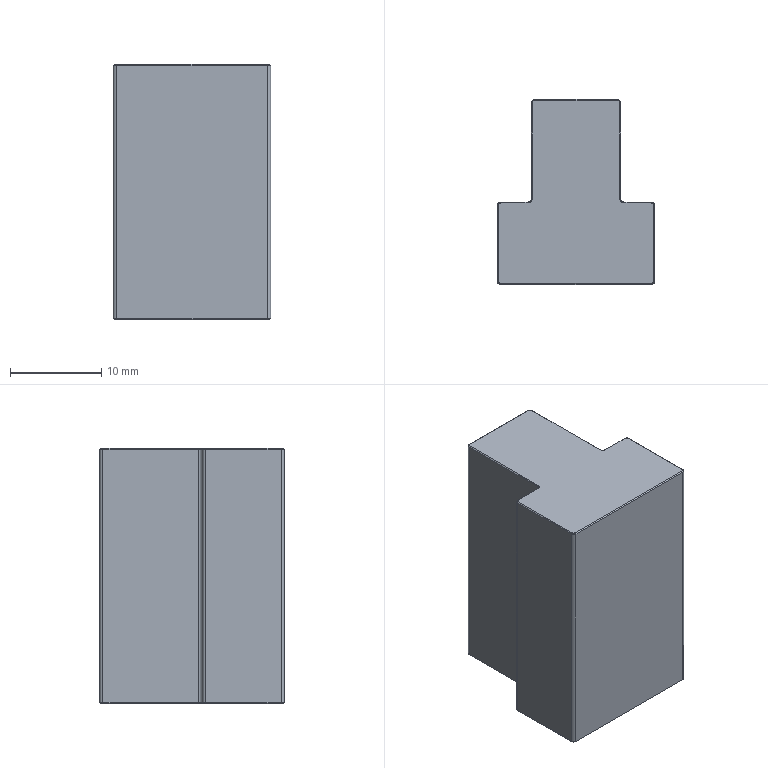Part | Creo | features DATUM PLANE 3, CHAMFER 1, COORDINATE SYSTEM 1, CURVE 1, PROTRUSION 1 | 1 solid | 50 faces | box 17.25 x 20.25 x 28 mm | volume 7414 mm3 | plane 26 | cone 16 | cylinder 8 | commonest cylinder face diameters 0.75 x8
STEP:
#1=CARTESIAN_POINT('',(0.,0.,0.));
#2=DIRECTION('',(0.,0.,1.));
#3=DIRECTION('',(1.,0.,0.));
#4=AXIS2_PLACEMENT_3D('',#1,#2,#3);
#5=CARTESIAN_POINT('',(-2.122,11.783,0.));
#6=VERTEX_POINT('',#5);
#7=CARTESIAN_POINT('',(-1.847,12.058,0.));
#8=VERTEX_POINT('',#7);
#9=CARTESIAN_POINT('',(-1.847,11.783,0.));
#10=DIRECTION('',(0.,0.,-1.));
#11=DIRECTION('',(-1.,0.,0.));
#12=AXIS2_PLACEMENT_3D('',#9,#10,#11);
#13=CIRCLE('',#12,0.275);
#14=EDGE_CURVE('',#6,#8,#13,.T.);
#15=ORIENTED_EDGE('',*,*,#14,.F.);
#16=CARTESIAN_POINT('',(-2.122,1.283,0.));
#17=VERTEX_POINT('',#16);
#18=CARTESIAN_POINT('',(-2.122,1.283,0.));
#19=DIRECTION('',(0.,1.,0.));
#20=VECTOR('',#19,10.5);
#21=LINE('',#18,#20);
#22=EDGE_CURVE('',#17,#6,#21,.T.);
#23=ORIENTED_EDGE('',*,*,#22,.F.);
#24=CARTESIAN_POINT('',(-2.597,0.8081,0.));
#25=VERTEX_POINT('',#24);
#26=CARTESIAN_POINT('',(-2.597,1.283,0.));
#27=DIRECTION('',(0.,0.,1.));
#28=DIRECTION('',(0.,-1.,0.));
#29=AXIS2_PLACEMENT_3D('',#26,#27,#28);
#30=CIRCLE('',#29,0.475);
#31=EDGE_CURVE('',#25,#17,#30,.T.);
#32=ORIENTED_EDGE('',*,*,#31,.F.);
#33=CARTESIAN_POINT('',(-5.597,0.8081,0.));
#34=VERTEX_POINT('',#33);
#35=CARTESIAN_POINT('',(-5.597,0.8081,-0.000000003));
#36=DIRECTION('',(1.,0.000000001,0.000000001));
#37=VECTOR('',#36,3.);
#38=LINE('',#35,#37);
#39=EDGE_CURVE('',#34,#25,#38,.T.);
#40=ORIENTED_EDGE('',*,*,#39,.F.);
#41=CARTESIAN_POINT('',(-5.872,0.5331,0.));
#42=VERTEX_POINT('',#41);
#43=CARTESIAN_POINT('',(-5.597,0.5331,0.));
#44=DIRECTION('',(0.,0.,-1.));
#45=DIRECTION('',(-1.,0.,0.));
#46=AXIS2_PLACEMENT_3D('',#43,#44,#45);
#47=CIRCLE('',#46,0.275);
#48=EDGE_CURVE('',#42,#34,#47,.T.);
#49=ORIENTED_EDGE('',*,*,#48,.F.);
#50=CARTESIAN_POINT('',(-5.872,-7.717,0.));
#51=VERTEX_POINT('',#50);
#52=CARTESIAN_POINT('',(-5.872,-7.717,-0.000000003));
#53=DIRECTION('',(0.,1.,0.));
#54=VECTOR('',#53,8.25);
#55=LINE('',#52,#54);
#56=EDGE_CURVE('',#51,#42,#55,.T.);
#57=ORIENTED_EDGE('',*,*,#56,.F.);
#58=CARTESIAN_POINT('',(-5.597,-7.992,0.));
#59=VERTEX_POINT('',#58);
#60=CARTESIAN_POINT('',(-5.597,-7.717,0.));
#61=DIRECTION('',(0.,0.,-1.));
#62=DIRECTION('',(0.,-1.,0.));
#63=AXIS2_PLACEMENT_3D('',#60,#61,#62);
#64=CIRCLE('',#63,0.275);
#65=EDGE_CURVE('',#59,#51,#64,.T.);
#66=ORIENTED_EDGE('',*,*,#65,.F.);
#67=CARTESIAN_POINT('',(10.903,-7.992,0.));
#68=VERTEX_POINT('',#67);
#69=CARTESIAN_POINT('',(10.903,-7.992,-0.000000003));
#70=DIRECTION('',(-1.,0.,0.));
#71=VECTOR('',#70,16.5);
#72=LINE('',#69,#71);
#73=EDGE_CURVE('',#68,#59,#72,.T.);
#74=ORIENTED_EDGE('',*,*,#73,.F.);
#75=CARTESIAN_POINT('',(11.178,-7.717,0.));
#76=VERTEX_POINT('',#75);
#77=CARTESIAN_POINT('',(10.903,-7.717,0.));
#78=DIRECTION('',(0.,0.,-1.));
#79=DIRECTION('',(1.,0.,0.));
#80=AXIS2_PLACEMENT_3D('',#77,#78,#79);
#81=CIRCLE('',#80,0.275);
#82=EDGE_CURVE('',#76,#68,#81,.T.);
#83=ORIENTED_EDGE('',*,*,#82,.F.);
#84=CARTESIAN_POINT('',(11.178,0.5331,0.));
#85=VERTEX_POINT('',#84);
#86=CARTESIAN_POINT('',(11.178,0.5331,-0.000000003));
#87=DIRECTION('',(0.,-1.,0.));
#88=VECTOR('',#87,8.25);
#89=LINE('',#86,#88);
#90=EDGE_CURVE('',#85,#76,#89,.T.);
#91=ORIENTED_EDGE('',*,*,#90,.F.);
#92=CARTESIAN_POINT('',(10.903,0.8081,0.));
#93=VERTEX_POINT('',#92);
#94=CARTESIAN_POINT('',(10.903,0.5331,0.));
#95=DIRECTION('',(0.,0.,-1.));
#96=DIRECTION('',(0.,1.,0.));
#97=AXIS2_PLACEMENT_3D('',#94,#95,#96);
#98=CIRCLE('',#97,0.275);
#99=EDGE_CURVE('',#93,#85,#98,.T.);
#100=ORIENTED_EDGE('',*,*,#99,.F.);
#101=CARTESIAN_POINT('',(7.903,0.8081,0.));
#102=VERTEX_POINT('',#101);
#103=CARTESIAN_POINT('',(7.903,0.8081,0.));
#104=DIRECTION('',(1.,0.,0.));
#105=VECTOR('',#104,3.);
#106=LINE('',#103,#105);
#107=EDGE_CURVE('',#102,#93,#106,.T.);
#108=ORIENTED_EDGE('',*,*,#107,.F.);
#109=CARTESIAN_POINT('',(7.428,1.283,0.));
#110=VERTEX_POINT('',#109);
#111=CARTESIAN_POINT('',(7.903,1.283,0.));
#112=DIRECTION('',(0.,0.,1.));
#113=DIRECTION('',(-1.,0.,0.));
#114=AXIS2_PLACEMENT_3D('',#111,#112,#113);
#115=CIRCLE('',#114,0.475);
#116=EDGE_CURVE('',#110,#102,#115,.T.);
#117=ORIENTED_EDGE('',*,*,#116,.F.);
#118=CARTESIAN_POINT('',(7.428,11.783,0.));
#119=VERTEX_POINT('',#118);
#120=CARTESIAN_POINT('',(7.428,11.783,-0.000000003));
#121=DIRECTION('',(0.,-1.,0.));
#122=VECTOR('',#121,10.5);
#123=LINE('',#120,#122);
#124=EDGE_CURVE('',#119,#110,#123,.T.);
#125=ORIENTED_EDGE('',*,*,#124,.F.);
#126=CARTESIAN_POINT('',(7.153,12.058,0.));
#127=VERTEX_POINT('',#126);
#128=CARTESIAN_POINT('',(7.153,11.783,0.));
#129=DIRECTION('',(0.,0.,-1.));
#130=DIRECTION('',(0.,1.,0.));
#131=AXIS2_PLACEMENT_3D('',#128,#129,#130);
#132=CIRCLE('',#131,0.275);
#133=EDGE_CURVE('',#127,#119,#132,.T.);
#134=ORIENTED_EDGE('',*,*,#133,.F.);
#135=CARTESIAN_POINT('',(-1.847,12.058,-0.000000003));
#136=DIRECTION('',(1.,0.,0.));
#137=VECTOR('',#136,9.);
#138=LINE('',#135,#137);
#139=EDGE_CURVE('',#8,#127,#138,.T.);
#140=ORIENTED_EDGE('',*,*,#139,.F.);
#141=EDGE_LOOP('',(#15,#23,#32,#40,#49,#57,#66,#74,#83,#91,#100,#108,#117,#125,#134,#140));
#142=FACE_OUTER_BOUND('',#141,.F.);
#143=CARTESIAN_POINT('',(0.,0.,0.));
#144=DIRECTION('',(0.,0.,1.));
#145=DIRECTION('',(1.,0.,0.));
#146=AXIS2_PLACEMENT_3D('',#143,#144,#145);
#147=PLANE('',#146);
#148=ADVANCED_FACE('',(#142),#147,.F.);
#149=ORIENTED_EDGE('',*,*,#14,.T.);
#150=CARTESIAN_POINT('',(-1.847,12.158,0.1));
#151=VERTEX_POINT('',#150);
#152=CARTESIAN_POINT('',(-1.847,12.058,-0.000000003));
#153=DIRECTION('',(-0.000000003,0.7071,0.7071));
#154=VECTOR('',#153,0.1414);
#155=LINE('',#152,#154);
#156=EDGE_CURVE('',#8,#151,#155,.T.);
#157=ORIENTED_EDGE('',*,*,#156,.T.);
#158=CARTESIAN_POINT('',(-2.222,11.783,0.1));
#159=VERTEX_POINT('',#158);
#160=CARTESIAN_POINT('',(-1.847,11.783,0.1));
#161=DIRECTION('',(0.,0.,-1.));
#162=DIRECTION('',(-1.,0.,0.));
#163=AXIS2_PLACEMENT_3D('',#160,#161,#162);
#164=CIRCLE('',#163,0.375);
#165=EDGE_CURVE('',#159,#151,#164,.T.);
#166=ORIENTED_EDGE('',*,*,#165,.F.);
#167=CARTESIAN_POINT('',(-2.122,11.783,0.));
#168=DIRECTION('',(-0.7071,0.000000001,0.7071));
#169=VECTOR('',#168,0.1414);
#170=LINE('',#167,#169);
#171=EDGE_CURVE('',#6,#159,#170,.T.);
#172=ORIENTED_EDGE('',*,*,#171,.F.);
#173=EDGE_LOOP('',(#149,#157,#166,#172));
#174=FACE_OUTER_BOUND('',#173,.F.);
#175=CARTESIAN_POINT('',(-1.847,11.783,0.05));
#176=DIRECTION('',(0.,0.,1.));
#177=DIRECTION('',(0.,-1.,0.));
#178=AXIS2_PLACEMENT_3D('',#175,#176,#177);
#179=CONICAL_SURFACE('',#178,0.325,45.);
#180=ADVANCED_FACE('',(#174),#179,.T.);
#181=ORIENTED_EDGE('',*,*,#139,.T.);
#182=CARTESIAN_POINT('',(7.153,12.158,0.1));
#183=VERTEX_POINT('',#182);
#184=CARTESIAN_POINT('',(7.153,12.058,0.));
#185=DIRECTION('',(0.000000001,0.7071,0.7071));
#186=VECTOR('',#185,0.1414);
#187=LINE('',#184,#186);
#188=EDGE_CURVE('',#127,#183,#187,.T.);
#189=ORIENTED_EDGE('',*,*,#188,.T.);
#190=CARTESIAN_POINT('',(-1.847,12.158,0.1));
#191=DIRECTION('',(1.,0.,0.));
#192=VECTOR('',#191,9.);
#193=LINE('',#190,#192);
#194=EDGE_CURVE('',#151,#183,#193,.T.);
#195=ORIENTED_EDGE('',*,*,#194,.F.);
#196=ORIENTED_EDGE('',*,*,#156,.F.);
#197=EDGE_LOOP('',(#181,#189,#195,#196));
#198=FACE_OUTER_BOUND('',#197,.F.);
#199=CARTESIAN_POINT('',(2.653,12.108,0.05));
#200=DIRECTION('',(0.,0.7071,-0.7071));
#201=DIRECTION('',(0.,0.7071,0.7071));
#202=AXIS2_PLACEMENT_3D('',#199,#200,#201);
#203=PLANE('',#202);
#204=ADVANCED_FACE('',(#198),#203,.T.);
#205=ORIENTED_EDGE('',*,*,#133,.T.);
#206=CARTESIAN_POINT('',(7.528,11.783,0.1));
#207=VERTEX_POINT('',#206);
#208=CARTESIAN_POINT('',(7.428,11.783,-0.000000003));
#209=DIRECTION('',(0.7071,0.000000003,0.7071));
#210=VECTOR('',#209,0.1414);
#211=LINE('',#208,#210);
#212=EDGE_CURVE('',#119,#207,#211,.T.);
#213=ORIENTED_EDGE('',*,*,#212,.T.);
#214=CARTESIAN_POINT('',(7.153,11.783,0.1));
#215=DIRECTION('',(0.,0.,-1.));
#216=DIRECTION('',(0.,1.,0.));
#217=AXIS2_PLACEMENT_3D('',#214,#215,#216);
#218=CIRCLE('',#217,0.375);
#219=EDGE_CURVE('',#183,#207,#218,.T.);
#220=ORIENTED_EDGE('',*,*,#219,.F.);
#221=ORIENTED_EDGE('',*,*,#188,.F.);
#222=EDGE_LOOP('',(#205,#213,#220,#221));
#223=FACE_OUTER_BOUND('',#222,.F.);
#224=CARTESIAN_POINT('',(7.153,11.783,0.05));
#225=DIRECTION('',(0.,0.,1.));
#226=DIRECTION('',(0.,-1.,0.));
#227=AXIS2_PLACEMENT_3D('',#224,#225,#226);
#228=CONICAL_SURFACE('',#227,0.325,45.);
#229=ADVANCED_FACE('',(#223),#228,.T.);
#230=ORIENTED_EDGE('',*,*,#124,.T.);
#231=CARTESIAN_POINT('',(7.528,1.283,0.1));
#232=VERTEX_POINT('',#231);
#233=CARTESIAN_POINT('',(7.428,1.283,0.));
#234=DIRECTION('',(0.7071,0.000000004,0.7071));
#235=VECTOR('',#234,0.1414);
#236=LINE('',#233,#235);
#237=EDGE_CURVE('',#110,#232,#236,.T.);
#238=ORIENTED_EDGE('',*,*,#237,.T.);
#239=CARTESIAN_POINT('',(7.528,11.783,0.1));
#240=DIRECTION('',(0.,-1.,0.));
#241=VECTOR('',#240,10.5);
#242=LINE('',#239,#241);
#243=EDGE_CURVE('',#207,#232,#242,.T.);
#244=ORIENTED_EDGE('',*,*,#243,.F.);
#245=ORIENTED_EDGE('',*,*,#212,.F.);
#246=EDGE_LOOP('',(#230,#238,#244,#245));
#247=FACE_OUTER_BOUND('',#246,.F.);
#248=CARTESIAN_POINT('',(7.478,6.533,0.05));
#249=DIRECTION('',(0.7071,0.,-0.7071));
#250=DIRECTION('',(0.7071,0.,0.7071));
#251=AXIS2_PLACEMENT_3D('',#248,#249,#250);
#252=PLANE('',#251);
#253=ADVANCED_FACE('',(#247),#252,.T.);
#254=ORIENTED_EDGE('',*,*,#116,.T.);
#255=CARTESIAN_POINT('',(7.903,0.9081,0.1));
#256=VERTEX_POINT('',#255);
#257=CARTESIAN_POINT('',(7.903,0.8081,0.));
#258=DIRECTION('',(0.000000005,0.7071,0.7071));
#259=VECTOR('',#258,0.1414);
#260=LINE('',#257,#259);
#261=EDGE_CURVE('',#102,#256,#260,.T.);
#262=ORIENTED_EDGE('',*,*,#261,.T.);
#263=CARTESIAN_POINT('',(7.903,1.283,0.1));
#264=DIRECTION('',(0.,0.,1.));
#265=DIRECTION('',(-1.,0.,0.));
#266=AXIS2_PLACEMENT_3D('',#263,#264,#265);
#267=CIRCLE('',#266,0.375);
#268=EDGE_CURVE('',#232,#256,#267,.T.);
#269=ORIENTED_EDGE('',*,*,#268,.F.);
#270=ORIENTED_EDGE('',*,*,#237,.F.);
#271=EDGE_LOOP('',(#254,#262,#269,#270));
#272=FACE_OUTER_BOUND('',#271,.F.);
#273=CARTESIAN_POINT('',(7.903,1.283,0.05));
#274=DIRECTION('',(0.,0.,-1.));
#275=DIRECTION('',(0.,-1.,0.));
#276=AXIS2_PLACEMENT_3D('',#273,#274,#275);
#277=CONICAL_SURFACE('',#276,0.425,45.);
#278=ADVANCED_FACE('',(#272),#277,.F.);
#279=ORIENTED_EDGE('',*,*,#107,.T.);
#280=CARTESIAN_POINT('',(10.903,0.9081,0.1));
#281=VERTEX_POINT('',#280);
#282=CARTESIAN_POINT('',(10.903,0.8081,0.));
#283=DIRECTION('',(0.000000001,0.7071,0.7071));
#284=VECTOR('',#283,0.1414);
#285=LINE('',#282,#284);
#286=EDGE_CURVE('',#93,#281,#285,.T.);
#287=ORIENTED_EDGE('',*,*,#286,.T.);
#288=CARTESIAN_POINT('',(7.903,0.9081,0.1));
#289=DIRECTION('',(1.,0.,0.));
#290=VECTOR('',#289,3.);
#291=LINE('',#288,#290);
#292=EDGE_CURVE('',#256,#281,#291,.T.);
#293=ORIENTED_EDGE('',*,*,#292,.F.);
#294=ORIENTED_EDGE('',*,*,#261,.F.);
#295=EDGE_LOOP('',(#279,#287,#293,#294));
#296=FACE_OUTER_BOUND('',#295,.F.);
#297=CARTESIAN_POINT('',(9.403,0.8581,0.05));
#298=DIRECTION('',(0.,0.7071,-0.7071));
#299=DIRECTION('',(0.,0.7071,0.7071));
#300=AXIS2_PLACEMENT_3D('',#297,#298,#299);
#301=PLANE('',#300);
#302=ADVANCED_FACE('',(#296),#301,.T.);
#303=ORIENTED_EDGE('',*,*,#99,.T.);
#304=CARTESIAN_POINT('',(11.278,0.5331,0.1));
#305=VERTEX_POINT('',#304);
#306=CARTESIAN_POINT('',(11.178,0.5331,-0.000000003));
#307=DIRECTION('',(0.7071,0.000000003,0.7071));
#308=VECTOR('',#307,0.1414);
#309=LINE('',#306,#308);
#310=EDGE_CURVE('',#85,#305,#309,.T.);
#311=ORIENTED_EDGE('',*,*,#310,.T.);
#312=CARTESIAN_POINT('',(10.903,0.5331,0.1));
#313=DIRECTION('',(0.,0.,-1.));
#314=DIRECTION('',(0.,1.,0.));
#315=AXIS2_PLACEMENT_3D('',#312,#313,#314);
#316=CIRCLE('',#315,0.375);
#317=EDGE_CURVE('',#281,#305,#316,.T.);
#318=ORIENTED_EDGE('',*,*,#317,.F.);
#319=ORIENTED_EDGE('',*,*,#286,.F.);
#320=EDGE_LOOP('',(#303,#311,#318,#319));
#321=FACE_OUTER_BOUND('',#320,.F.);
#322=CARTESIAN_POINT('',(10.903,0.5331,0.05));
#323=DIRECTION('',(0.,0.,1.));
#324=DIRECTION('',(0.,-1.,0.));
#325=AXIS2_PLACEMENT_3D('',#322,#323,#324);
#326=CONICAL_SURFACE('',#325,0.325,45.);
#327=ADVANCED_FACE('',(#321),#326,.T.);
#328=ORIENTED_EDGE('',*,*,#90,.T.);
#329=CARTESIAN_POINT('',(11.278,-7.717,0.1));
#330=VERTEX_POINT('',#329);
#331=CARTESIAN_POINT('',(11.178,-7.717,0.));
#332=DIRECTION('',(0.7071,-0.000000001,0.7071));
#333=VECTOR('',#332,0.1414);
#334=LINE('',#331,#333);
#335=EDGE_CURVE('',#76,#330,#334,.T.);
#336=ORIENTED_EDGE('',*,*,#335,.T.);
#337=CARTESIAN_POINT('',(11.278,0.5331,0.1));
#338=DIRECTION('',(0.,-1.,0.));
#339=VECTOR('',#338,8.25);
#340=LINE('',#337,#339);
#341=EDGE_CURVE('',#305,#330,#340,.T.);
#342=ORIENTED_EDGE('',*,*,#341,.F.);
#343=ORIENTED_EDGE('',*,*,#310,.F.);
#344=EDGE_LOOP('',(#328,#336,#342,#343));
#345=FACE_OUTER_BOUND('',#344,.F.);
#346=CARTESIAN_POINT('',(11.228,-3.592,0.05));
#347=DIRECTION('',(0.7071,0.,-0.7071));
#348=DIRECTION('',(0.7071,0.,0.7071));
#349=AXIS2_PLACEMENT_3D('',#346,#347,#348);
#350=PLANE('',#349);
#351=ADVANCED_FACE('',(#345),#350,.T.);
#352=ORIENTED_EDGE('',*,*,#82,.T.);
#353=CARTESIAN_POINT('',(10.903,-8.092,0.1));
#354=VERTEX_POINT('',#353);
#355=CARTESIAN_POINT('',(10.903,-7.992,-0.000000003));
#356=DIRECTION('',(0.000000003,-0.7071,0.7071));
#357=VECTOR('',#356,0.1414);
#358=LINE('',#355,#357);
#359=EDGE_CURVE('',#68,#354,#358,.T.);
#360=ORIENTED_EDGE('',*,*,#359,.T.);
#361=CARTESIAN_POINT('',(10.903,-7.717,0.1));
#362=DIRECTION('',(0.,0.,-1.));
#363=DIRECTION('',(1.,0.,0.));
#364=AXIS2_PLACEMENT_3D('',#361,#362,#363);
#365=CIRCLE('',#364,0.375);
#366=EDGE_CURVE('',#330,#354,#365,.T.);
#367=ORIENTED_EDGE('',*,*,#366,.F.);
#368=ORIENTED_EDGE('',*,*,#335,.F.);
#369=EDGE_LOOP('',(#352,#360,#367,#368));
#370=FACE_OUTER_BOUND('',#369,.F.);
#371=CARTESIAN_POINT('',(10.903,-7.717,0.05));
#372=DIRECTION('',(0.,0.,1.));
#373=DIRECTION('',(0.,-1.,0.));
#374=AXIS2_PLACEMENT_3D('',#371,#372,#373);
#375=CONICAL_SURFACE('',#374,0.325,45.);
#376=ADVANCED_FACE('',(#370),#375,.T.);
#377=ORIENTED_EDGE('',*,*,#73,.T.);
#378=CARTESIAN_POINT('',(-5.597,-8.092,0.1));
#379=VERTEX_POINT('',#378);
#380=CARTESIAN_POINT('',(-5.597,-7.992,0.));
#381=DIRECTION('',(-0.000000001,-0.7071,0.7071));
#382=VECTOR('',#381,0.1414);
#383=LINE('',#380,#382);
#384=EDGE_CURVE('',#59,#379,#383,.T.);
#385=ORIENTED_EDGE('',*,*,#384,.T.);
#386=CARTESIAN_POINT('',(10.903,-8.092,0.1));
#387=DIRECTION('',(-1.,0.,0.));
#388=VECTOR('',#387,16.5);
#389=LINE('',#386,#388);
#390=EDGE_CURVE('',#354,#379,#389,.T.);
#391=ORIENTED_EDGE('',*,*,#390,.F.);
#392=ORIENTED_EDGE('',*,*,#359,.F.);
#393=EDGE_LOOP('',(#377,#385,#391,#392));
#394=FACE_OUTER_BOUND('',#393,.F.);
#395=CARTESIAN_POINT('',(2.653,-8.042,0.05));
#396=DIRECTION('',(0.,-0.7071,-0.7071));
#397=DIRECTION('',(0.,-0.7071,0.7071));
#398=AXIS2_PLACEMENT_3D('',#395,#396,#397);
#399=PLANE('',#398);
#400=ADVANCED_FACE('',(#394),#399,.T.);
#401=ORIENTED_EDGE('',*,*,#65,.T.);
#402=CARTESIAN_POINT('',(-5.972,-7.717,0.1));
#403=VERTEX_POINT('',#402);
#404=CARTESIAN_POINT('',(-5.872,-7.717,-0.000000003));
#405=DIRECTION('',(-0.7071,-0.000000003,0.7071));
#406=VECTOR('',#405,0.1414);
#407=LINE('',#404,#406);
#408=EDGE_CURVE('',#51,#403,#407,.T.);
#409=ORIENTED_EDGE('',*,*,#408,.T.);
#410=CARTESIAN_POINT('',(-5.597,-7.717,0.1));
#411=DIRECTION('',(0.,0.,-1.));
#412=DIRECTION('',(0.,-1.,0.));
#413=AXIS2_PLACEMENT_3D('',#410,#411,#412);
#414=CIRCLE('',#413,0.375);
#415=EDGE_CURVE('',#379,#403,#414,.T.);
#416=ORIENTED_EDGE('',*,*,#415,.F.);
#417=ORIENTED_EDGE('',*,*,#384,.F.);
#418=EDGE_LOOP('',(#401,#409,#416,#417));
#419=FACE_OUTER_BOUND('',#418,.F.);
#420=CARTESIAN_POINT('',(-5.597,-7.717,0.05));
#421=DIRECTION('',(0.,0.,1.));
#422=DIRECTION('',(0.,-1.,0.));
#423=AXIS2_PLACEMENT_3D('',#420,#421,#422);
#424=CONICAL_SURFACE('',#423,0.325,45.);
#425=ADVANCED_FACE('',(#419),#424,.T.);
#426=ORIENTED_EDGE('',*,*,#56,.T.);
#427=CARTESIAN_POINT('',(-5.972,0.5331,0.1));
#428=VERTEX_POINT('',#427);
#429=CARTESIAN_POINT('',(-5.872,0.5331,0.));
#430=DIRECTION('',(-0.7071,0.000000001,0.7071));
#431=VECTOR('',#430,0.1414);
#432=LINE('',#429,#431);
#433=EDGE_CURVE('',#42,#428,#432,.T.);
#434=ORIENTED_EDGE('',*,*,#433,.T.);
#435=CARTESIAN_POINT('',(-5.972,-7.717,0.1));
#436=DIRECTION('',(0.,1.,0.));
#437=VECTOR('',#436,8.25);
#438=LINE('',#435,#437);
#439=EDGE_CURVE('',#403,#428,#438,.T.);
#440=ORIENTED_EDGE('',*,*,#439,.F.);
#441=ORIENTED_EDGE('',*,*,#408,.F.);
#442=EDGE_LOOP('',(#426,#434,#440,#441));
#443=FACE_OUTER_BOUND('',#442,.F.);
#444=CARTESIAN_POINT('',(-5.922,-3.592,0.05));
#445=DIRECTION('',(-0.7071,0.,-0.7071));
#446=DIRECTION('',(-0.7071,0.,0.7071));
#447=AXIS2_PLACEMENT_3D('',#444,#445,#446);
#448=PLANE('',#447);
#449=ADVANCED_FACE('',(#443),#448,.T.);
#450=ORIENTED_EDGE('',*,*,#48,.T.);
#451=CARTESIAN_POINT('',(-5.597,0.9081,0.1));
#452=VERTEX_POINT('',#451);
#453=CARTESIAN_POINT('',(-5.597,0.8081,-0.000000003));
#454=DIRECTION('',(-0.000000003,0.7071,0.7071));
#455=VECTOR('',#454,0.1414);
#456=LINE('',#453,#455);
#457=EDGE_CURVE('',#34,#452,#456,.T.);
#458=ORIENTED_EDGE('',*,*,#457,.T.);
#459=CARTESIAN_POINT('',(-5.597,0.5331,0.1));
#460=DIRECTION('',(0.,0.,-1.));
#461=DIRECTION('',(-1.,0.,0.));
#462=AXIS2_PLACEMENT_3D('',#459,#460,#461);
#463=CIRCLE('',#462,0.375);
#464=EDGE_CURVE('',#428,#452,#463,.T.);
#465=ORIENTED_EDGE('',*,*,#464,.F.);
#466=ORIENTED_EDGE('',*,*,#433,.F.);
#467=EDGE_LOOP('',(#450,#458,#465,#466));
#468=FACE_OUTER_BOUND('',#467,.F.);
#469=CARTESIAN_POINT('',(-5.597,0.5331,0.05));
#470=DIRECTION('',(0.,0.,1.));
#471=DIRECTION('',(0.,-1.,0.));
#472=AXIS2_PLACEMENT_3D('',#469,#470,#471);
#473=CONICAL_SURFACE('',#472,0.325,45.);
#474=ADVANCED_FACE('',(#468),#473,.T.);
#475=ORIENTED_EDGE('',*,*,#39,.T.);
#476=CARTESIAN_POINT('',(-2.597,0.9081,0.1));
#477=VERTEX_POINT('',#476);
#478=CARTESIAN_POINT('',(-2.597,0.8081,0.));
#479=DIRECTION('',(-0.000000004,0.7071,0.7071));
#480=VECTOR('',#479,0.1414);
#481=LINE('',#478,#480);
#482=EDGE_CURVE('',#25,#477,#481,.T.);
#483=ORIENTED_EDGE('',*,*,#482,.T.);
#484=CARTESIAN_POINT('',(-5.597,0.9081,0.1));
#485=DIRECTION('',(1.,0.000000001,0.000000001));
#486=VECTOR('',#485,3.);
#487=LINE('',#484,#486);
#488=EDGE_CURVE('',#452,#477,#487,.T.);
#489=ORIENTED_EDGE('',*,*,#488,.F.);
#490=ORIENTED_EDGE('',*,*,#457,.F.);
#491=EDGE_LOOP('',(#475,#483,#489,#490));
#492=FACE_OUTER_BOUND('',#491,.F.);
#493=CARTESIAN_POINT('',(-4.097,0.8581,0.05));
#494=DIRECTION('',(0.,0.7071,-0.7071));
#495=DIRECTION('',(0.,0.7071,0.7071));
#496=AXIS2_PLACEMENT_3D('',#493,#494,#495);
#497=PLANE('',#496);
#498=ADVANCED_FACE('',(#492),#497,.T.);
#499=ORIENTED_EDGE('',*,*,#31,.T.);
#500=CARTESIAN_POINT('',(-2.222,1.283,0.1));
#501=VERTEX_POINT('',#500);
#502=CARTESIAN_POINT('',(-2.122,1.283,0.));
#503=DIRECTION('',(-0.7071,0.000000005,0.7071));
#504=VECTOR('',#503,0.1414);
#505=LINE('',#502,#504);
#506=EDGE_CURVE('',#17,#501,#505,.T.);
#507=ORIENTED_EDGE('',*,*,#506,.T.);
#508=CARTESIAN_POINT('',(-2.597,1.283,0.1));
#509=DIRECTION('',(0.,0.,1.));
#510=DIRECTION('',(0.,-1.,0.));
#511=AXIS2_PLACEMENT_3D('',#508,#509,#510);
#512=CIRCLE('',#511,0.375);
#513=EDGE_CURVE('',#477,#501,#512,.T.);
#514=ORIENTED_EDGE('',*,*,#513,.F.);
#515=ORIENTED_EDGE('',*,*,#482,.F.);
#516=EDGE_LOOP('',(#499,#507,#514,#515));
#517=FACE_OUTER_BOUND('',#516,.F.);
#518=CARTESIAN_POINT('',(-2.597,1.283,0.05));
#519=DIRECTION('',(0.,0.,-1.));
#520=DIRECTION('',(0.,-1.,0.));
#521=AXIS2_PLACEMENT_3D('',#518,#519,#520);
#522=CONICAL_SURFACE('',#521,0.425,45.);
#523=ADVANCED_FACE('',(#517),#522,.F.);
#524=ORIENTED_EDGE('',*,*,#22,.T.);
#525=ORIENTED_EDGE('',*,*,#171,.T.);
#526=CARTESIAN_POINT('',(-2.222,1.283,0.1));
#527=DIRECTION('',(0.,1.,0.));
#528=VECTOR('',#527,10.5);
#529=LINE('',#526,#528);
#530=EDGE_CURVE('',#501,#159,#529,.T.);
#531=ORIENTED_EDGE('',*,*,#530,.F.);
#532=ORIENTED_EDGE('',*,*,#506,.F.);
#533=EDGE_LOOP('',(#524,#525,#531,#532));
#534=FACE_OUTER_BOUND('',#533,.F.);
#535=CARTESIAN_POINT('',(-2.172,6.533,0.05));
#536=DIRECTION('',(-0.7071,0.,-0.7071));
#537=DIRECTION('',(-0.7071,0.,0.7071));
#538=AXIS2_PLACEMENT_3D('',#535,#536,#537);
#539=PLANE('',#538);
#540=ADVANCED_FACE('',(#534),#539,.T.);
#541=CARTESIAN_POINT('',(-2.222,11.783,27.9));
#542=VERTEX_POINT('',#541);
#543=CARTESIAN_POINT('',(-2.222,1.283,27.9));
#544=VERTEX_POINT('',#543);
#545=CARTESIAN_POINT('',(-2.222,11.783,27.9));
#546=DIRECTION('',(0.,-1.,0.));
#547=VECTOR('',#546,10.5);
#548=LINE('',#545,#547);
#549=EDGE_CURVE('',#542,#544,#548,.T.);
#550=ORIENTED_EDGE('',*,*,#549,.T.);
#551=CARTESIAN_POINT('',(-2.222,1.283,0.1));
#552=DIRECTION('',(0.,0.,1.));
#553=VECTOR('',#552,27.8);
#554=LINE('',#551,#553);
#555=EDGE_CURVE('',#501,#544,#554,.T.);
#556=ORIENTED_EDGE('',*,*,#555,.F.);
#557=ORIENTED_EDGE('',*,*,#530,.T.);
#558=CARTESIAN_POINT('',(-2.222,11.783,0.1));
#559=DIRECTION('',(0.,0.,1.));
#560=VECTOR('',#559,27.8);
#561=LINE('',#558,#560);
#562=EDGE_CURVE('',#159,#542,#561,.T.);
#563=ORIENTED_EDGE('',*,*,#562,.T.);
#564=EDGE_LOOP('',(#550,#556,#557,#563));
#565=FACE_OUTER_BOUND('',#564,.F.);
#566=CARTESIAN_POINT('',(-2.222,11.783,0.));
#567=DIRECTION('',(-1.,0.,0.));
#568=DIRECTION('',(0.,-1.,0.));
#569=AXIS2_PLACEMENT_3D('',#566,#567,#568);
#570=PLANE('',#569);
#571=ADVANCED_FACE('',(#565),#570,.T.);
#572=CARTESIAN_POINT('',(-2.122,11.783,28.));
#573=VERTEX_POINT('',#572);
#574=CARTESIAN_POINT('',(-2.122,1.283,28.));
#575=VERTEX_POINT('',#574);
#576=CARTESIAN_POINT('',(-2.122,11.783,28.));
#577=DIRECTION('',(0.,-1.,0.));
#578=VECTOR('',#577,10.5);
#579=LINE('',#576,#578);
#580=EDGE_CURVE('',#573,#575,#579,.T.);
#581=ORIENTED_EDGE('',*,*,#580,.T.);
#582=CARTESIAN_POINT('',(-2.122,1.283,28.));
#583=DIRECTION('',(-0.7071,0.000000005,-0.7071));
#584=VECTOR('',#583,0.1414);
#585=LINE('',#582,#584);
#586=EDGE_CURVE('',#575,#544,#585,.T.);
#587=ORIENTED_EDGE('',*,*,#586,.T.);
#588=ORIENTED_EDGE('',*,*,#549,.F.);
#589=CARTESIAN_POINT('',(-2.122,11.783,28.));
#590=DIRECTION('',(-0.7071,0.000000001,-0.7071));
#591=VECTOR('',#590,0.1414);
#592=LINE('',#589,#591);
#593=EDGE_CURVE('',#573,#542,#592,.T.);
#594=ORIENTED_EDGE('',*,*,#593,.F.);
#595=EDGE_LOOP('',(#581,#587,#588,#594));
#596=FACE_OUTER_BOUND('',#595,.F.);
#597=CARTESIAN_POINT('',(-2.172,6.533,27.95));
#598=DIRECTION('',(-0.7071,0.,0.7071));
#599=DIRECTION('',(-0.7071,0.,-0.7071));
#600=AXIS2_PLACEMENT_3D('',#597,#598,#599);
#601=PLANE('',#600);
#602=ADVANCED_FACE('',(#596),#601,.T.);
#603=CARTESIAN_POINT('',(-2.597,0.8081,28.));
#604=VERTEX_POINT('',#603);
#605=CARTESIAN_POINT('',(-2.597,1.283,28.));
#606=DIRECTION('',(0.,0.,-1.));
#607=DIRECTION('',(1.,0.,0.));
#608=AXIS2_PLACEMENT_3D('',#605,#606,#607);
#609=CIRCLE('',#608,0.475);
#610=EDGE_CURVE('',#575,#604,#609,.T.);
#611=ORIENTED_EDGE('',*,*,#610,.F.);
#612=ORIENTED_EDGE('',*,*,#580,.F.);
#613=CARTESIAN_POINT('',(-1.847,12.058,28.));
#614=VERTEX_POINT('',#613);
#615=CARTESIAN_POINT('',(-1.847,11.783,28.));
#616=DIRECTION('',(0.,0.,1.));
#617=DIRECTION('',(0.,1.,0.));
#618=AXIS2_PLACEMENT_3D('',#615,#616,#617);
#619=CIRCLE('',#618,0.275);
#620=EDGE_CURVE('',#614,#573,#619,.T.);
#621=ORIENTED_EDGE('',*,*,#620,.F.);
#622=CARTESIAN_POINT('',(7.153,12.058,28.));
#623=VERTEX_POINT('',#622);
#624=CARTESIAN_POINT('',(7.153,12.058,28.));
#625=DIRECTION('',(-1.,0.,0.));
#626=VECTOR('',#625,9.);
#627=LINE('',#624,#626);
#628=EDGE_CURVE('',#623,#614,#627,.T.);
#629=ORIENTED_EDGE('',*,*,#628,.F.);
#630=CARTESIAN_POINT('',(7.428,11.783,28.));
#631=VERTEX_POINT('',#630);
#632=CARTESIAN_POINT('',(7.153,11.783,28.));
#633=DIRECTION('',(0.,0.,1.));
#634=DIRECTION('',(1.,0.,0.));
#635=AXIS2_PLACEMENT_3D('',#632,#633,#634);
#636=CIRCLE('',#635,0.275);
#637=EDGE_CURVE('',#631,#623,#636,.T.);
#638=ORIENTED_EDGE('',*,*,#637,.F.);
#639=CARTESIAN_POINT('',(7.428,1.283,28.));
#640=VERTEX_POINT('',#639);
#641=CARTESIAN_POINT('',(7.428,1.283,28.));
#642=DIRECTION('',(0.,1.,0.));
#643=VECTOR('',#642,10.5);
#644=LINE('',#641,#643);
#645=EDGE_CURVE('',#640,#631,#644,.T.);
#646=ORIENTED_EDGE('',*,*,#645,.F.);
#647=CARTESIAN_POINT('',(7.903,0.8081,28.));
#648=VERTEX_POINT('',#647);
#649=CARTESIAN_POINT('',(7.903,1.283,28.));
#650=DIRECTION('',(0.,0.,-1.));
#651=DIRECTION('',(0.,-1.,0.));
#652=AXIS2_PLACEMENT_3D('',#649,#650,#651);
#653=CIRCLE('',#652,0.475);
#654=EDGE_CURVE('',#648,#640,#653,.T.);
#655=ORIENTED_EDGE('',*,*,#654,.F.);
#656=CARTESIAN_POINT('',(10.903,0.8081,28.));
#657=VERTEX_POINT('',#656);
#658=CARTESIAN_POINT('',(10.903,0.8081,28.));
#659=DIRECTION('',(-1.,0.,0.));
#660=VECTOR('',#659,3.);
#661=LINE('',#658,#660);
#662=EDGE_CURVE('',#657,#648,#661,.T.);
#663=ORIENTED_EDGE('',*,*,#662,.F.);
#664=CARTESIAN_POINT('',(11.178,0.5331,28.));
#665=VERTEX_POINT('',#664);
#666=CARTESIAN_POINT('',(10.903,0.5331,28.));
#667=DIRECTION('',(0.,0.,1.));
#668=DIRECTION('',(1.,0.,0.));
#669=AXIS2_PLACEMENT_3D('',#666,#667,#668);
#670=CIRCLE('',#669,0.275);
#671=EDGE_CURVE('',#665,#657,#670,.T.);
#672=ORIENTED_EDGE('',*,*,#671,.F.);
#673=CARTESIAN_POINT('',(11.178,-7.717,28.));
#674=VERTEX_POINT('',#673);
#675=CARTESIAN_POINT('',(11.178,-7.717,28.));
#676=DIRECTION('',(0.,1.,0.));
#677=VECTOR('',#676,8.25);
#678=LINE('',#675,#677);
#679=EDGE_CURVE('',#674,#665,#678,.T.);
#680=ORIENTED_EDGE('',*,*,#679,.F.);
#681=CARTESIAN_POINT('',(10.903,-7.992,28.));
#682=VERTEX_POINT('',#681);
#683=CARTESIAN_POINT('',(10.903,-7.717,28.));
#684=DIRECTION('',(0.,0.,1.));
#685=DIRECTION('',(0.,-1.,0.));
#686=AXIS2_PLACEMENT_3D('',#683,#684,#685);
#687=CIRCLE('',#686,0.275);
#688=EDGE_CURVE('',#682,#674,#687,.T.);
#689=ORIENTED_EDGE('',*,*,#688,.F.);
#690=CARTESIAN_POINT('',(-5.597,-7.992,28.));
#691=VERTEX_POINT('',#690);
#692=CARTESIAN_POINT('',(-5.597,-7.992,28.));
#693=DIRECTION('',(1.,0.,0.));
#694=VECTOR('',#693,16.5);
#695=LINE('',#692,#694);
#696=EDGE_CURVE('',#691,#682,#695,.T.);
#697=ORIENTED_EDGE('',*,*,#696,.F.);
#698=CARTESIAN_POINT('',(-5.872,-7.717,28.));
#699=VERTEX_POINT('',#698);
#700=CARTESIAN_POINT('',(-5.597,-7.717,28.));
#701=DIRECTION('',(0.,0.,1.));
#702=DIRECTION('',(-1.,0.,0.));
#703=AXIS2_PLACEMENT_3D('',#700,#701,#702);
#704=CIRCLE('',#703,0.275);
#705=EDGE_CURVE('',#699,#691,#704,.T.);
#706=ORIENTED_EDGE('',*,*,#705,.F.);
#707=CARTESIAN_POINT('',(-5.872,0.5331,28.));
#708=VERTEX_POINT('',#707);
#709=CARTESIAN_POINT('',(-5.872,0.5331,28.));
#710=DIRECTION('',(0.,-1.,0.));
#711=VECTOR('',#710,8.25);
#712=LINE('',#709,#711);
#713=EDGE_CURVE('',#708,#699,#712,.T.);
#714=ORIENTED_EDGE('',*,*,#713,.F.);
#715=CARTESIAN_POINT('',(-5.597,0.8081,28.));
#716=VERTEX_POINT('',#715);
#717=CARTESIAN_POINT('',(-5.597,0.5331,28.));
#718=DIRECTION('',(0.,0.,1.));
#719=DIRECTION('',(0.,1.,0.));
#720=AXIS2_PLACEMENT_3D('',#717,#718,#719);
#721=CIRCLE('',#720,0.275);
#722=EDGE_CURVE('',#716,#708,#721,.T.);
#723=ORIENTED_EDGE('',*,*,#722,.F.);
#724=CARTESIAN_POINT('',(-2.597,0.8081,28.));
#725=DIRECTION('',(-1.,-0.000000001,0.000000001));
#726=VECTOR('',#725,3.);
#727=LINE('',#724,#726);
#728=EDGE_CURVE('',#604,#716,#727,.T.);
#729=ORIENTED_EDGE('',*,*,#728,.F.);
#730=EDGE_LOOP('',(#611,#612,#621,#629,#638,#646,#655,#663,#672,#680,#689,#697,#706,#714,#723,#729));
#731=FACE_OUTER_BOUND('',#730,.F.);
#732=CARTESIAN_POINT('',(0.,0.,28.));
#733=DIRECTION('',(0.,0.,1.));
#734=DIRECTION('',(1.,0.,0.));
#735=AXIS2_PLACEMENT_3D('',#732,#733,#734);
#736=PLANE('',#735);
#737=ADVANCED_FACE('',(#731),#736,.T.);
#738=ORIENTED_EDGE('',*,*,#610,.T.);
#739=CARTESIAN_POINT('',(-2.597,0.9081,27.9));
#740=VERTEX_POINT('',#739);
#741=CARTESIAN_POINT('',(-2.597,0.8081,28.));
#742=DIRECTION('',(-0.000000004,0.7071,-0.7071));
#743=VECTOR('',#742,0.1414);
#744=LINE('',#741,#743);
#745=EDGE_CURVE('',#604,#740,#744,.T.);
#746=ORIENTED_EDGE('',*,*,#745,.T.);
#747=CARTESIAN_POINT('',(-2.597,1.283,27.9));
#748=DIRECTION('',(0.,0.,-1.));
#749=DIRECTION('',(1.,0.,0.));
#750=AXIS2_PLACEMENT_3D('',#747,#748,#749);
#751=CIRCLE('',#750,0.375);
#752=EDGE_CURVE('',#544,#740,#751,.T.);
#753=ORIENTED_EDGE('',*,*,#752,.F.);
#754=ORIENTED_EDGE('',*,*,#586,.F.);
#755=EDGE_LOOP('',(#738,#746,#753,#754));
#756=FACE_OUTER_BOUND('',#755,.F.);
#757=CARTESIAN_POINT('',(-2.597,1.283,27.95));
#758=DIRECTION('',(0.,0.,1.));
#759=DIRECTION('',(0.,-1.,0.));
#760=AXIS2_PLACEMENT_3D('',#757,#758,#759);
#761=CONICAL_SURFACE('',#760,0.425,45.);
#762=ADVANCED_FACE('',(#756),#761,.F.);
#763=ORIENTED_EDGE('',*,*,#728,.T.);
#764=CARTESIAN_POINT('',(-5.597,0.9081,27.9));
#765=VERTEX_POINT('',#764);
#766=CARTESIAN_POINT('',(-5.597,0.8081,28.));
#767=DIRECTION('',(-0.000000003,0.7071,-0.7071));
#768=VECTOR('',#767,0.1414);
#769=LINE('',#766,#768);
#770=EDGE_CURVE('',#716,#765,#769,.T.);
#771=ORIENTED_EDGE('',*,*,#770,.T.);
#772=CARTESIAN_POINT('',(-2.597,0.9081,27.9));
#773=DIRECTION('',(-1.,-0.000000001,0.000000001));
#774=VECTOR('',#773,3.);
#775=LINE('',#772,#774);
#776=EDGE_CURVE('',#740,#765,#775,.T.);
#777=ORIENTED_EDGE('',*,*,#776,.F.);
#778=ORIENTED_EDGE('',*,*,#745,.F.);
#779=EDGE_LOOP('',(#763,#771,#777,#778));
#780=FACE_OUTER_BOUND('',#779,.F.);
#781=CARTESIAN_POINT('',(-4.097,0.8581,27.95));
#782=DIRECTION('',(0.,0.7071,0.7071));
#783=DIRECTION('',(0.,0.7071,-0.7071));
#784=AXIS2_PLACEMENT_3D('',#781,#782,#783);
#785=PLANE('',#784);
#786=ADVANCED_FACE('',(#780),#785,.T.);
#787=ORIENTED_EDGE('',*,*,#722,.T.);
#788=CARTESIAN_POINT('',(-5.972,0.5331,27.9));
#789=VERTEX_POINT('',#788);
#790=CARTESIAN_POINT('',(-5.872,0.5331,28.));
#791=DIRECTION('',(-0.7071,0.000000001,-0.7071));
#792=VECTOR('',#791,0.1414);
#793=LINE('',#790,#792);
#794=EDGE_CURVE('',#708,#789,#793,.T.);
#795=ORIENTED_EDGE('',*,*,#794,.T.);
#796=CARTESIAN_POINT('',(-5.597,0.5331,27.9));
#797=DIRECTION('',(0.,0.,1.));
#798=DIRECTION('',(0.,1.,0.));
#799=AXIS2_PLACEMENT_3D('',#796,#797,#798);
#800=CIRCLE('',#799,0.375);
#801=EDGE_CURVE('',#765,#789,#800,.T.);
#802=ORIENTED_EDGE('',*,*,#801,.F.);
#803=ORIENTED_EDGE('',*,*,#770,.F.);
#804=EDGE_LOOP('',(#787,#795,#802,#803));
#805=FACE_OUTER_BOUND('',#804,.F.);
#806=CARTESIAN_POINT('',(-5.597,0.5331,27.95));
#807=DIRECTION('',(0.,0.,-1.));
#808=DIRECTION('',(0.,-1.,0.));
#809=AXIS2_PLACEMENT_3D('',#806,#807,#808);
#810=CONICAL_SURFACE('',#809,0.325,45.);
#811=ADVANCED_FACE('',(#805),#810,.T.);
#812=ORIENTED_EDGE('',*,*,#713,.T.);
#813=CARTESIAN_POINT('',(-5.972,-7.717,27.9));
#814=VERTEX_POINT('',#813);
#815=CARTESIAN_POINT('',(-5.872,-7.717,28.));
#816=DIRECTION('',(-0.7071,-0.000000003,-0.7071));
#817=VECTOR('',#816,0.1414);
#818=LINE('',#815,#817);
#819=EDGE_CURVE('',#699,#814,#818,.T.);
#820=ORIENTED_EDGE('',*,*,#819,.T.);
#821=CARTESIAN_POINT('',(-5.972,0.5331,27.9));
#822=DIRECTION('',(0.,-1.,0.));
#823=VECTOR('',#822,8.25);
#824=LINE('',#821,#823);
#825=EDGE_CURVE('',#789,#814,#824,.T.);
#826=ORIENTED_EDGE('',*,*,#825,.F.);
#827=ORIENTED_EDGE('',*,*,#794,.F.);
#828=EDGE_LOOP('',(#812,#820,#826,#827));
#829=FACE_OUTER_BOUND('',#828,.F.);
#830=CARTESIAN_POINT('',(-5.922,-3.592,27.95));
#831=DIRECTION('',(-0.7071,0.,0.7071));
#832=DIRECTION('',(-0.7071,0.,-0.7071));
#833=AXIS2_PLACEMENT_3D('',#830,#831,#832);
#834=PLANE('',#833);
#835=ADVANCED_FACE('',(#829),#834,.T.);
#836=ORIENTED_EDGE('',*,*,#705,.T.);
#837=CARTESIAN_POINT('',(-5.597,-8.092,27.9));
#838=VERTEX_POINT('',#837);
#839=CARTESIAN_POINT('',(-5.597,-7.992,28.));
#840=DIRECTION('',(-0.000000001,-0.7071,-0.7071));
#841=VECTOR('',#840,0.1414);
#842=LINE('',#839,#841);
#843=EDGE_CURVE('',#691,#838,#842,.T.);
#844=ORIENTED_EDGE('',*,*,#843,.T.);
#845=CARTESIAN_POINT('',(-5.597,-7.717,27.9));
#846=DIRECTION('',(0.,0.,1.));
#847=DIRECTION('',(-1.,0.,0.));
#848=AXIS2_PLACEMENT_3D('',#845,#846,#847);
#849=CIRCLE('',#848,0.375);
#850=EDGE_CURVE('',#814,#838,#849,.T.);
#851=ORIENTED_EDGE('',*,*,#850,.F.);
#852=ORIENTED_EDGE('',*,*,#819,.F.);
#853=EDGE_LOOP('',(#836,#844,#851,#852));
#854=FACE_OUTER_BOUND('',#853,.F.);
#855=CARTESIAN_POINT('',(-5.597,-7.717,27.95));
#856=DIRECTION('',(0.,0.,-1.));
#857=DIRECTION('',(0.,-1.,0.));
#858=AXIS2_PLACEMENT_3D('',#855,#856,#857);
#859=CONICAL_SURFACE('',#858,0.325,45.);
#860=ADVANCED_FACE('',(#854),#859,.T.);
#861=ORIENTED_EDGE('',*,*,#696,.T.);
#862=CARTESIAN_POINT('',(10.903,-8.092,27.9));
#863=VERTEX_POINT('',#862);
#864=CARTESIAN_POINT('',(10.903,-7.992,28.));
#865=DIRECTION('',(0.000000003,-0.7071,-0.7071));
#866=VECTOR('',#865,0.1414);
#867=LINE('',#864,#866);
#868=EDGE_CURVE('',#682,#863,#867,.T.);
#869=ORIENTED_EDGE('',*,*,#868,.T.);
#870=CARTESIAN_POINT('',(-5.597,-8.092,27.9));
#871=DIRECTION('',(1.,0.,0.));
#872=VECTOR('',#871,16.5);
#873=LINE('',#870,#872);
#874=EDGE_CURVE('',#838,#863,#873,.T.);
#875=ORIENTED_EDGE('',*,*,#874,.F.);
#876=ORIENTED_EDGE('',*,*,#843,.F.);
#877=EDGE_LOOP('',(#861,#869,#875,#876));
#878=FACE_OUTER_BOUND('',#877,.F.);
#879=CARTESIAN_POINT('',(2.653,-8.042,27.95));
#880=DIRECTION('',(0.,-0.7071,0.7071));
#881=DIRECTION('',(0.,-0.7071,-0.7071));
#882=AXIS2_PLACEMENT_3D('',#879,#880,#881);
#883=PLANE('',#882);
#884=ADVANCED_FACE('',(#878),#883,.T.);
#885=ORIENTED_EDGE('',*,*,#688,.T.);
#886=CARTESIAN_POINT('',(11.278,-7.717,27.9));
#887=VERTEX_POINT('',#886);
#888=CARTESIAN_POINT('',(11.178,-7.717,28.));
#889=DIRECTION('',(0.7071,-0.000000001,-0.7071));
#890=VECTOR('',#889,0.1414);
#891=LINE('',#888,#890);
#892=EDGE_CURVE('',#674,#887,#891,.T.);
#893=ORIENTED_EDGE('',*,*,#892,.T.);
#894=CARTESIAN_POINT('',(10.903,-7.717,27.9));
#895=DIRECTION('',(0.,0.,1.));
#896=DIRECTION('',(0.,-1.,0.));
#897=AXIS2_PLACEMENT_3D('',#894,#895,#896);
#898=CIRCLE('',#897,0.375);
#899=EDGE_CURVE('',#863,#887,#898,.T.);
#900=ORIENTED_EDGE('',*,*,#899,.F.);
#901=ORIENTED_EDGE('',*,*,#868,.F.);
#902=EDGE_LOOP('',(#885,#893,#900,#901));
#903=FACE_OUTER_BOUND('',#902,.F.);
#904=CARTESIAN_POINT('',(10.903,-7.717,27.95));
#905=DIRECTION('',(0.,0.,-1.));
#906=DIRECTION('',(0.,-1.,0.));
#907=AXIS2_PLACEMENT_3D('',#904,#905,#906);
#908=CONICAL_SURFACE('',#907,0.325,45.);
#909=ADVANCED_FACE('',(#903),#908,.T.);
#910=ORIENTED_EDGE('',*,*,#679,.T.);
#911=CARTESIAN_POINT('',(11.278,0.5331,27.9));
#912=VERTEX_POINT('',#911);
#913=CARTESIAN_POINT('',(11.178,0.5331,28.));
#914=DIRECTION('',(0.7071,0.000000003,-0.7071));
#915=VECTOR('',#914,0.1414);
#916=LINE('',#913,#915);
#917=EDGE_CURVE('',#665,#912,#916,.T.);
#918=ORIENTED_EDGE('',*,*,#917,.T.);
#919=CARTESIAN_POINT('',(11.278,-7.717,27.9));
#920=DIRECTION('',(0.,1.,0.));
#921=VECTOR('',#920,8.25);
#922=LINE('',#919,#921);
#923=EDGE_CURVE('',#887,#912,#922,.T.);
#924=ORIENTED_EDGE('',*,*,#923,.F.);
#925=ORIENTED_EDGE('',*,*,#892,.F.);
#926=EDGE_LOOP('',(#910,#918,#924,#925));
#927=FACE_OUTER_BOUND('',#926,.F.);
#928=CARTESIAN_POINT('',(11.228,-3.592,27.95));
#929=DIRECTION('',(0.7071,0.,0.7071));
#930=DIRECTION('',(0.7071,0.,-0.7071));
#931=AXIS2_PLACEMENT_3D('',#928,#929,#930);
#932=PLANE('',#931);
#933=ADVANCED_FACE('',(#927),#932,.T.);
#934=ORIENTED_EDGE('',*,*,#671,.T.);
#935=CARTESIAN_POINT('',(10.903,0.9081,27.9));
#936=VERTEX_POINT('',#935);
#937=CARTESIAN_POINT('',(10.903,0.8081,28.));
#938=DIRECTION('',(0.000000001,0.7071,-0.7071));
#939=VECTOR('',#938,0.1414);
#940=LINE('',#937,#939);
#941=EDGE_CURVE('',#657,#936,#940,.T.);
#942=ORIENTED_EDGE('',*,*,#941,.T.);
#943=CARTESIAN_POINT('',(10.903,0.5331,27.9));
#944=DIRECTION('',(0.,0.,1.));
#945=DIRECTION('',(1.,0.,0.));
#946=AXIS2_PLACEMENT_3D('',#943,#944,#945);
#947=CIRCLE('',#946,0.375);
#948=EDGE_CURVE('',#912,#936,#947,.T.);
#949=ORIENTED_EDGE('',*,*,#948,.F.);
#950=ORIENTED_EDGE('',*,*,#917,.F.);
#951=EDGE_LOOP('',(#934,#942,#949,#950));
#952=FACE_OUTER_BOUND('',#951,.F.);
#953=CARTESIAN_POINT('',(10.903,0.5331,27.95));
#954=DIRECTION('',(0.,0.,-1.));
#955=DIRECTION('',(0.,-1.,0.));
#956=AXIS2_PLACEMENT_3D('',#953,#954,#955);
#957=CONICAL_SURFACE('',#956,0.325,45.);
#958=ADVANCED_FACE('',(#952),#957,.T.);
#959=ORIENTED_EDGE('',*,*,#662,.T.);
#960=CARTESIAN_POINT('',(7.903,0.9081,27.9));
#961=VERTEX_POINT('',#960);
#962=CARTESIAN_POINT('',(7.903,0.8081,28.));
#963=DIRECTION('',(0.000000005,0.7071,-0.7071));
#964=VECTOR('',#963,0.1414);
#965=LINE('',#962,#964);
#966=EDGE_CURVE('',#648,#961,#965,.T.);
#967=ORIENTED_EDGE('',*,*,#966,.T.);
#968=CARTESIAN_POINT('',(10.903,0.9081,27.9));
#969=DIRECTION('',(-1.,0.,0.));
#970=VECTOR('',#969,3.);
#971=LINE('',#968,#970);
#972=EDGE_CURVE('',#936,#961,#971,.T.);
#973=ORIENTED_EDGE('',*,*,#972,.F.);
#974=ORIENTED_EDGE('',*,*,#941,.F.);
#975=EDGE_LOOP('',(#959,#967,#973,#974));
#976=FACE_OUTER_BOUND('',#975,.F.);
#977=CARTESIAN_POINT('',(9.403,0.8581,27.95));
#978=DIRECTION('',(0.,0.7071,0.7071));
#979=DIRECTION('',(0.,0.7071,-0.7071));
#980=AXIS2_PLACEMENT_3D('',#977,#978,#979);
#981=PLANE('',#980);
#982=ADVANCED_FACE('',(#976),#981,.T.);
#983=ORIENTED_EDGE('',*,*,#654,.T.);
#984=CARTESIAN_POINT('',(7.528,1.283,27.9));
#985=VERTEX_POINT('',#984);
#986=CARTESIAN_POINT('',(7.428,1.283,28.));
#987=DIRECTION('',(0.7071,0.000000004,-0.7071));
#988=VECTOR('',#987,0.1414);
#989=LINE('',#986,#988);
#990=EDGE_CURVE('',#640,#985,#989,.T.);
#991=ORIENTED_EDGE('',*,*,#990,.T.);
#992=CARTESIAN_POINT('',(7.903,1.283,27.9));
#993=DIRECTION('',(0.,0.,-1.));
#994=DIRECTION('',(0.,-1.,0.));
#995=AXIS2_PLACEMENT_3D('',#992,#993,#994);
#996=CIRCLE('',#995,0.375);
#997=EDGE_CURVE('',#961,#985,#996,.T.);
#998=ORIENTED_EDGE('',*,*,#997,.F.);
#999=ORIENTED_EDGE('',*,*,#966,.F.);
#1000=EDGE_LOOP('',(#983,#991,#998,#999));
#1001=FACE_OUTER_BOUND('',#1000,.F.);
#1002=CARTESIAN_POINT('',(7.903,1.283,27.95));
#1003=DIRECTION('',(0.,0.,1.));
#1004=DIRECTION('',(0.,-1.,0.));
#1005=AXIS2_PLACEMENT_3D('',#1002,#1003,#1004);
#1006=CONICAL_SURFACE('',#1005,0.425,45.);
#1007=ADVANCED_FACE('',(#1001),#1006,.F.);
#1008=ORIENTED_EDGE('',*,*,#645,.T.);
#1009=CARTESIAN_POINT('',(7.528,11.783,27.9));
#1010=VERTEX_POINT('',#1009);
#1011=CARTESIAN_POINT('',(7.428,11.783,28.));
#1012=DIRECTION('',(0.7071,0.000000003,-0.7071));
#1013=VECTOR('',#1012,0.1414);
#1014=LINE('',#1011,#1013);
#1015=EDGE_CURVE('',#631,#1010,#1014,.T.);
#1016=ORIENTED_EDGE('',*,*,#1015,.T.);
#1017=CARTESIAN_POINT('',(7.528,1.283,27.9));
#1018=DIRECTION('',(0.,1.,0.));
#1019=VECTOR('',#1018,10.5);
#1020=LINE('',#1017,#1019);
#1021=EDGE_CURVE('',#985,#1010,#1020,.T.);
#1022=ORIENTED_EDGE('',*,*,#1021,.F.);
#1023=ORIENTED_EDGE('',*,*,#990,.F.);
#1024=EDGE_LOOP('',(#1008,#1016,#1022,#1023));
#1025=FACE_OUTER_BOUND('',#1024,.F.);
#1026=CARTESIAN_POINT('',(7.478,6.533,27.95));
#1027=DIRECTION('',(0.7071,0.,0.7071));
#1028=DIRECTION('',(0.7071,0.,-0.7071));
#1029=AXIS2_PLACEMENT_3D('',#1026,#1027,#1028);
#1030=PLANE('',#1029);
#1031=ADVANCED_FACE('',(#1025),#1030,.T.);
#1032=ORIENTED_EDGE('',*,*,#637,.T.);
#1033=CARTESIAN_POINT('',(7.153,12.158,27.9));
#1034=VERTEX_POINT('',#1033);
#1035=CARTESIAN_POINT('',(7.153,12.058,28.));
#1036=DIRECTION('',(0.000000001,0.7071,-0.7071));
#1037=VECTOR('',#1036,0.1414);
#1038=LINE('',#1035,#1037);
#1039=EDGE_CURVE('',#623,#1034,#1038,.T.);
#1040=ORIENTED_EDGE('',*,*,#1039,.T.);
#1041=CARTESIAN_POINT('',(7.153,11.783,27.9));
#1042=DIRECTION('',(0.,0.,1.));
#1043=DIRECTION('',(1.,0.,0.));
#1044=AXIS2_PLACEMENT_3D('',#1041,#1042,#1043);
#1045=CIRCLE('',#1044,0.375);
#1046=EDGE_CURVE('',#1010,#1034,#1045,.T.);
#1047=ORIENTED_EDGE('',*,*,#1046,.F.);
#1048=ORIENTED_EDGE('',*,*,#1015,.F.);
#1049=EDGE_LOOP('',(#1032,#1040,#1047,#1048));
#1050=FACE_OUTER_BOUND('',#1049,.F.);
#1051=CARTESIAN_POINT('',(7.153,11.783,27.95));
#1052=DIRECTION('',(0.,0.,-1.));
#1053=DIRECTION('',(0.,-1.,0.));
#1054=AXIS2_PLACEMENT_3D('',#1051,#1052,#1053);
#1055=CONICAL_SURFACE('',#1054,0.325,45.);
#1056=ADVANCED_FACE('',(#1050),#1055,.T.);
#1057=ORIENTED_EDGE('',*,*,#628,.T.);
#1058=CARTESIAN_POINT('',(-1.847,12.158,27.9));
#1059=VERTEX_POINT('',#1058);
#1060=CARTESIAN_POINT('',(-1.847,12.058,28.));
#1061=DIRECTION('',(-0.000000003,0.7071,-0.7071));
#1062=VECTOR('',#1061,0.1414);
#1063=LINE('',#1060,#1062);
#1064=EDGE_CURVE('',#614,#1059,#1063,.T.);
#1065=ORIENTED_EDGE('',*,*,#1064,.T.);
#1066=CARTESIAN_POINT('',(7.153,12.158,27.9));
#1067=DIRECTION('',(-1.,0.,0.));
#1068=VECTOR('',#1067,9.);
#1069=LINE('',#1066,#1068);
#1070=EDGE_CURVE('',#1034,#1059,#1069,.T.);
#1071=ORIENTED_EDGE('',*,*,#1070,.F.);
#1072=ORIENTED_EDGE('',*,*,#1039,.F.);
#1073=EDGE_LOOP('',(#1057,#1065,#1071,#1072));
#1074=FACE_OUTER_BOUND('',#1073,.F.);
#1075=CARTESIAN_POINT('',(2.653,12.108,27.95));
#1076=DIRECTION('',(0.,0.7071,0.7071));
#1077=DIRECTION('',(0.,0.7071,-0.7071));
#1078=AXIS2_PLACEMENT_3D('',#1075,#1076,#1077);
#1079=PLANE('',#1078);
#1080=ADVANCED_FACE('',(#1074),#1079,.T.);
#1081=ORIENTED_EDGE('',*,*,#620,.T.);
#1082=ORIENTED_EDGE('',*,*,#593,.T.);
#1083=CARTESIAN_POINT('',(-1.847,11.783,27.9));
#1084=DIRECTION('',(0.,0.,1.));
#1085=DIRECTION('',(0.,1.,0.));
#1086=AXIS2_PLACEMENT_3D('',#1083,#1084,#1085);
#1087=CIRCLE('',#1086,0.375);
#1088=EDGE_CURVE('',#1059,#542,#1087,.T.);
#1089=ORIENTED_EDGE('',*,*,#1088,.F.);
#1090=ORIENTED_EDGE('',*,*,#1064,.F.);
#1091=EDGE_LOOP('',(#1081,#1082,#1089,#1090));
#1092=FACE_OUTER_BOUND('',#1091,.F.);
#1093=CARTESIAN_POINT('',(-1.847,11.783,27.95));
#1094=DIRECTION('',(0.,0.,-1.));
#1095=DIRECTION('',(0.,-1.,0.));
#1096=AXIS2_PLACEMENT_3D('',#1093,#1094,#1095);
#1097=CONICAL_SURFACE('',#1096,0.325,45.);
#1098=ADVANCED_FACE('',(#1092),#1097,.T.);
#1099=ORIENTED_EDGE('',*,*,#1088,.T.);
#1100=ORIENTED_EDGE('',*,*,#562,.F.);
#1101=ORIENTED_EDGE('',*,*,#165,.T.);
#1102=CARTESIAN_POINT('',(-1.847,12.158,0.1));
#1103=DIRECTION('',(0.,0.,1.));
#1104=VECTOR('',#1103,27.8);
#1105=LINE('',#1102,#1104);
#1106=EDGE_CURVE('',#151,#1059,#1105,.T.);
#1107=ORIENTED_EDGE('',*,*,#1106,.T.);
#1108=EDGE_LOOP('',(#1099,#1100,#1101,#1107));
#1109=FACE_OUTER_BOUND('',#1108,.F.);
#1110=CARTESIAN_POINT('',(-1.847,11.783,0.));
#1111=DIRECTION('',(0.,0.,1.));
#1112=DIRECTION('',(1.,0.,0.));
#1113=AXIS2_PLACEMENT_3D('',#1110,#1111,#1112);
#1114=CYLINDRICAL_SURFACE('',#1113,0.375);
#1115=ADVANCED_FACE('',(#1109),#1114,.T.);
#1116=ORIENTED_EDGE('',*,*,#1070,.T.);
#1117=ORIENTED_EDGE('',*,*,#1106,.F.);
#1118=ORIENTED_EDGE('',*,*,#194,.T.);
#1119=CARTESIAN_POINT('',(7.153,12.158,0.1));
#1120=DIRECTION('',(0.,0.,1.));
#1121=VECTOR('',#1120,27.8);
#1122=LINE('',#1119,#1121);
#1123=EDGE_CURVE('',#183,#1034,#1122,.T.);
#1124=ORIENTED_EDGE('',*,*,#1123,.T.);
#1125=EDGE_LOOP('',(#1116,#1117,#1118,#1124));
#1126=FACE_OUTER_BOUND('',#1125,.F.);
#1127=CARTESIAN_POINT('',(7.153,12.158,0.));
#1128=DIRECTION('',(0.,1.,0.));
#1129=DIRECTION('',(-1.,0.,0.));
#1130=AXIS2_PLACEMENT_3D('',#1127,#1128,#1129);
#1131=PLANE('',#1130);
#1132=ADVANCED_FACE('',(#1126),#1131,.T.);
#1133=ORIENTED_EDGE('',*,*,#1046,.T.);
#1134=ORIENTED_EDGE('',*,*,#1123,.F.);
#1135=ORIENTED_EDGE('',*,*,#219,.T.);
#1136=CARTESIAN_POINT('',(7.528,11.783,0.1));
#1137=DIRECTION('',(0.,0.,1.));
#1138=VECTOR('',#1137,27.8);
#1139=LINE('',#1136,#1138);
#1140=EDGE_CURVE('',#207,#1010,#1139,.T.);
#1141=ORIENTED_EDGE('',*,*,#1140,.T.);
#1142=EDGE_LOOP('',(#1133,#1134,#1135,#1141));
#1143=FACE_OUTER_BOUND('',#1142,.F.);
#1144=CARTESIAN_POINT('',(7.153,11.783,0.));
#1145=DIRECTION('',(0.,0.,1.));
#1146=DIRECTION('',(1.,0.,0.));
#1147=AXIS2_PLACEMENT_3D('',#1144,#1145,#1146);
#1148=CYLINDRICAL_SURFACE('',#1147,0.375);
#1149=ADVANCED_FACE('',(#1143),#1148,.T.);
#1150=ORIENTED_EDGE('',*,*,#1021,.T.);
#1151=ORIENTED_EDGE('',*,*,#1140,.F.);
#1152=ORIENTED_EDGE('',*,*,#243,.T.);
#1153=CARTESIAN_POINT('',(7.528,1.283,0.1));
#1154=DIRECTION('',(0.,0.,1.));
#1155=VECTOR('',#1154,27.8);
#1156=LINE('',#1153,#1155);
#1157=EDGE_CURVE('',#232,#985,#1156,.T.);
#1158=ORIENTED_EDGE('',*,*,#1157,.T.);
#1159=EDGE_LOOP('',(#1150,#1151,#1152,#1158));
#1160=FACE_OUTER_BOUND('',#1159,.F.);
#1161=CARTESIAN_POINT('',(7.528,1.283,0.));
#1162=DIRECTION('',(1.,0.,0.));
#1163=DIRECTION('',(0.,1.,0.));
#1164=AXIS2_PLACEMENT_3D('',#1161,#1162,#1163);
#1165=PLANE('',#1164);
#1166=ADVANCED_FACE('',(#1160),#1165,.T.);
#1167=ORIENTED_EDGE('',*,*,#997,.T.);
#1168=ORIENTED_EDGE('',*,*,#1157,.F.);
#1169=ORIENTED_EDGE('',*,*,#268,.T.);
#1170=CARTESIAN_POINT('',(7.903,0.9081,0.1));
#1171=DIRECTION('',(0.,0.,1.));
#1172=VECTOR('',#1171,27.8);
#1173=LINE('',#1170,#1172);
#1174=EDGE_CURVE('',#256,#961,#1173,.T.);
#1175=ORIENTED_EDGE('',*,*,#1174,.T.);
#1176=EDGE_LOOP('',(#1167,#1168,#1169,#1175));
#1177=FACE_OUTER_BOUND('',#1176,.F.);
#1178=CARTESIAN_POINT('',(7.903,1.283,0.));
#1179=DIRECTION('',(0.,0.,1.));
#1180=DIRECTION('',(1.,0.,0.));
#1181=AXIS2_PLACEMENT_3D('',#1178,#1179,#1180);
#1182=CYLINDRICAL_SURFACE('',#1181,0.375);
#1183=ADVANCED_FACE('',(#1177),#1182,.F.);
#1184=ORIENTED_EDGE('',*,*,#972,.T.);
#1185=ORIENTED_EDGE('',*,*,#1174,.F.);
#1186=ORIENTED_EDGE('',*,*,#292,.T.);
#1187=CARTESIAN_POINT('',(10.903,0.9081,0.1));
#1188=DIRECTION('',(0.,0.,1.));
#1189=VECTOR('',#1188,27.8);
#1190=LINE('',#1187,#1189);
#1191=EDGE_CURVE('',#281,#936,#1190,.T.);
#1192=ORIENTED_EDGE('',*,*,#1191,.T.);
#1193=EDGE_LOOP('',(#1184,#1185,#1186,#1192));
#1194=FACE_OUTER_BOUND('',#1193,.F.);
#1195=CARTESIAN_POINT('',(10.903,0.9081,0.));
#1196=DIRECTION('',(0.,1.,0.));
#1197=DIRECTION('',(-1.,0.,0.));
#1198=AXIS2_PLACEMENT_3D('',#1195,#1196,#1197);
#1199=PLANE('',#1198);
#1200=ADVANCED_FACE('',(#1194),#1199,.T.);
#1201=ORIENTED_EDGE('',*,*,#948,.T.);
#1202=ORIENTED_EDGE('',*,*,#1191,.F.);
#1203=ORIENTED_EDGE('',*,*,#317,.T.);
#1204=CARTESIAN_POINT('',(11.278,0.5331,0.1));
#1205=DIRECTION('',(0.,0.,1.));
#1206=VECTOR('',#1205,27.8);
#1207=LINE('',#1204,#1206);
#1208=EDGE_CURVE('',#305,#912,#1207,.T.);
#1209=ORIENTED_EDGE('',*,*,#1208,.T.);
#1210=EDGE_LOOP('',(#1201,#1202,#1203,#1209));
#1211=FACE_OUTER_BOUND('',#1210,.F.);
#1212=CARTESIAN_POINT('',(10.903,0.5331,0.));
#1213=DIRECTION('',(0.,0.,1.));
#1214=DIRECTION('',(1.,0.,0.));
#1215=AXIS2_PLACEMENT_3D('',#1212,#1213,#1214);
#1216=CYLINDRICAL_SURFACE('',#1215,0.375);
#1217=ADVANCED_FACE('',(#1211),#1216,.T.);
#1218=ORIENTED_EDGE('',*,*,#923,.T.);
#1219=ORIENTED_EDGE('',*,*,#1208,.F.);
#1220=ORIENTED_EDGE('',*,*,#341,.T.);
#1221=CARTESIAN_POINT('',(11.278,-7.717,0.1));
#1222=DIRECTION('',(0.,0.,1.));
#1223=VECTOR('',#1222,27.8);
#1224=LINE('',#1221,#1223);
#1225=EDGE_CURVE('',#330,#887,#1224,.T.);
#1226=ORIENTED_EDGE('',*,*,#1225,.T.);
#1227=EDGE_LOOP('',(#1218,#1219,#1220,#1226));
#1228=FACE_OUTER_BOUND('',#1227,.F.);
#1229=CARTESIAN_POINT('',(11.278,-7.717,0.));
#1230=DIRECTION('',(1.,0.,0.));
#1231=DIRECTION('',(0.,1.,0.));
#1232=AXIS2_PLACEMENT_3D('',#1229,#1230,#1231);
#1233=PLANE('',#1232);
#1234=ADVANCED_FACE('',(#1228),#1233,.T.);
#1235=ORIENTED_EDGE('',*,*,#899,.T.);
#1236=ORIENTED_EDGE('',*,*,#1225,.F.);
#1237=ORIENTED_EDGE('',*,*,#366,.T.);
#1238=CARTESIAN_POINT('',(10.903,-8.092,0.1));
#1239=DIRECTION('',(0.,0.,1.));
#1240=VECTOR('',#1239,27.8);
#1241=LINE('',#1238,#1240);
#1242=EDGE_CURVE('',#354,#863,#1241,.T.);
#1243=ORIENTED_EDGE('',*,*,#1242,.T.);
#1244=EDGE_LOOP('',(#1235,#1236,#1237,#1243));
#1245=FACE_OUTER_BOUND('',#1244,.F.);
#1246=CARTESIAN_POINT('',(10.903,-7.717,0.));
#1247=DIRECTION('',(0.,0.,1.));
#1248=DIRECTION('',(1.,0.,0.));
#1249=AXIS2_PLACEMENT_3D('',#1246,#1247,#1248);
#1250=CYLINDRICAL_SURFACE('',#1249,0.375);
#1251=ADVANCED_FACE('',(#1245),#1250,.T.);
#1252=ORIENTED_EDGE('',*,*,#874,.T.);
#1253=ORIENTED_EDGE('',*,*,#1242,.F.);
#1254=ORIENTED_EDGE('',*,*,#390,.T.);
#1255=CARTESIAN_POINT('',(-5.597,-8.092,0.1));
#1256=DIRECTION('',(0.,0.,1.));
#1257=VECTOR('',#1256,27.8);
#1258=LINE('',#1255,#1257);
#1259=EDGE_CURVE('',#379,#838,#1258,.T.);
#1260=ORIENTED_EDGE('',*,*,#1259,.T.);
#1261=EDGE_LOOP('',(#1252,#1253,#1254,#1260));
#1262=FACE_OUTER_BOUND('',#1261,.F.);
#1263=CARTESIAN_POINT('',(-5.597,-8.092,0.));
#1264=DIRECTION('',(0.,-1.,0.));
#1265=DIRECTION('',(1.,0.,0.));
#1266=AXIS2_PLACEMENT_3D('',#1263,#1264,#1265);
#1267=PLANE('',#1266);
#1268=ADVANCED_FACE('',(#1262),#1267,.T.);
#1269=ORIENTED_EDGE('',*,*,#850,.T.);
#1270=ORIENTED_EDGE('',*,*,#1259,.F.);
#1271=ORIENTED_EDGE('',*,*,#415,.T.);
#1272=CARTESIAN_POINT('',(-5.972,-7.717,0.1));
#1273=DIRECTION('',(0.,0.,1.));
#1274=VECTOR('',#1273,27.8);
#1275=LINE('',#1272,#1274);
#1276=EDGE_CURVE('',#403,#814,#1275,.T.);
#1277=ORIENTED_EDGE('',*,*,#1276,.T.);
#1278=EDGE_LOOP('',(#1269,#1270,#1271,#1277));
#1279=FACE_OUTER_BOUND('',#1278,.F.);
#1280=CARTESIAN_POINT('',(-5.597,-7.717,0.));
#1281=DIRECTION('',(0.,0.,1.));
#1282=DIRECTION('',(1.,0.,0.));
#1283=AXIS2_PLACEMENT_3D('',#1280,#1281,#1282);
#1284=CYLINDRICAL_SURFACE('',#1283,0.375);
#1285=ADVANCED_FACE('',(#1279),#1284,.T.);
#1286=ORIENTED_EDGE('',*,*,#825,.T.);
#1287=ORIENTED_EDGE('',*,*,#1276,.F.);
#1288=ORIENTED_EDGE('',*,*,#439,.T.);
#1289=CARTESIAN_POINT('',(-5.972,0.5331,0.1));
#1290=DIRECTION('',(0.,0.,1.));
#1291=VECTOR('',#1290,27.8);
#1292=LINE('',#1289,#1291);
#1293=EDGE_CURVE('',#428,#789,#1292,.T.);
#1294=ORIENTED_EDGE('',*,*,#1293,.T.);
#1295=EDGE_LOOP('',(#1286,#1287,#1288,#1294));
#1296=FACE_OUTER_BOUND('',#1295,.F.);
#1297=CARTESIAN_POINT('',(-5.972,0.5331,0.));
#1298=DIRECTION('',(-1.,0.,0.));
#1299=DIRECTION('',(0.,-1.,0.));
#1300=AXIS2_PLACEMENT_3D('',#1297,#1298,#1299);
#1301=PLANE('',#1300);
#1302=ADVANCED_FACE('',(#1296),#1301,.T.);
#1303=ORIENTED_EDGE('',*,*,#801,.T.);
#1304=ORIENTED_EDGE('',*,*,#1293,.F.);
#1305=ORIENTED_EDGE('',*,*,#464,.T.);
#1306=CARTESIAN_POINT('',(-5.597,0.9081,0.1));
#1307=DIRECTION('',(0.,0.,1.));
#1308=VECTOR('',#1307,27.8);
#1309=LINE('',#1306,#1308);
#1310=EDGE_CURVE('',#452,#765,#1309,.T.);
#1311=ORIENTED_EDGE('',*,*,#1310,.T.);
#1312=EDGE_LOOP('',(#1303,#1304,#1305,#1311));
#1313=FACE_OUTER_BOUND('',#1312,.F.);
#1314=CARTESIAN_POINT('',(-5.597,0.5331,0.));
#1315=DIRECTION('',(0.,0.,1.));
#1316=DIRECTION('',(1.,0.,0.));
#1317=AXIS2_PLACEMENT_3D('',#1314,#1315,#1316);
#1318=CYLINDRICAL_SURFACE('',#1317,0.375);
#1319=ADVANCED_FACE('',(#1313),#1318,.T.);
#1320=ORIENTED_EDGE('',*,*,#776,.T.);
#1321=ORIENTED_EDGE('',*,*,#1310,.F.);
#1322=ORIENTED_EDGE('',*,*,#488,.T.);
#1323=CARTESIAN_POINT('',(-2.597,0.9081,0.1));
#1324=DIRECTION('',(0.,0.,1.));
#1325=VECTOR('',#1324,27.8);
#1326=LINE('',#1323,#1325);
#1327=EDGE_CURVE('',#477,#740,#1326,.T.);
#1328=ORIENTED_EDGE('',*,*,#1327,.T.);
#1329=EDGE_LOOP('',(#1320,#1321,#1322,#1328));
#1330=FACE_OUTER_BOUND('',#1329,.F.);
#1331=CARTESIAN_POINT('',(-2.597,0.9081,0.));
#1332=DIRECTION('',(0.,1.,0.));
#1333=DIRECTION('',(-1.,0.,0.));
#1334=AXIS2_PLACEMENT_3D('',#1331,#1332,#1333);
#1335=PLANE('',#1334);
#1336=ADVANCED_FACE('',(#1330),#1335,.T.);
#1337=ORIENTED_EDGE('',*,*,#752,.T.);
#1338=ORIENTED_EDGE('',*,*,#1327,.F.);
#1339=ORIENTED_EDGE('',*,*,#513,.T.);
#1340=ORIENTED_EDGE('',*,*,#555,.T.);
#1341=EDGE_LOOP('',(#1337,#1338,#1339,#1340));
#1342=FACE_OUTER_BOUND('',#1341,.F.);
#1343=CARTESIAN_POINT('',(-2.597,1.283,0.));
#1344=DIRECTION('',(0.,0.,1.));
#1345=DIRECTION('',(1.,0.,0.));
#1346=AXIS2_PLACEMENT_3D('',#1343,#1344,#1345);
#1347=CYLINDRICAL_SURFACE('',#1346,0.375);
#1348=ADVANCED_FACE('',(#1342),#1347,.F.);
#1349=CLOSED_SHELL('',(#148,#180,#204,#229,#253,#278,#302,#327,#351,#376,#400,#425,#449,#474,#498,#523,#540,#571,#602,#737,#762,#786,#811,#835,#860,#884,#909,#933,#958,#982,#1007,#1031,#1056,#1080,#1098,#1115,#1132,#1149,#1166,#1183,#1200,#1217,#1234,#1251,#1268,#1285,#1302,#1319,#1336,#1348));
#1350=MANIFOLD_SOLID_BREP('',#1349);
#1351=(LENGTH_UNIT()NAMED_UNIT(*)SI_UNIT(.MILLI.,.METRE.));
#1352=UNCERTAINTY_MEASURE_WITH_UNIT(LENGTH_MEASURE(0.003862),#1351,'','');
#1353=(NAMED_UNIT(*)PLANE_ANGLE_UNIT()SI_UNIT($,.RADIAN.));
#1354=PLANE_ANGLE_MEASURE_WITH_UNIT(PLANE_ANGLE_MEASURE(0.01745),#1353);
#1355=(CONVERSION_BASED_UNIT('DEGREE',#1354)NAMED_UNIT(*)PLANE_ANGLE_UNIT());
#1356=(NAMED_UNIT(*)SI_UNIT($,.STERADIAN.)SOLID_ANGLE_UNIT());
#1357=(GEOMETRIC_REPRESENTATION_CONTEXT(3)GLOBAL_UNCERTAINTY_ASSIGNED_CONTEXT((#1352))GLOBAL_UNIT_ASSIGNED_CONTEXT((#1351,#1355,#1356))REPRESENTATION_CONTEXT('',''));
#1358=ADVANCED_BREP_SHAPE_REPRESENTATION('',(#4,#1350),#1357);